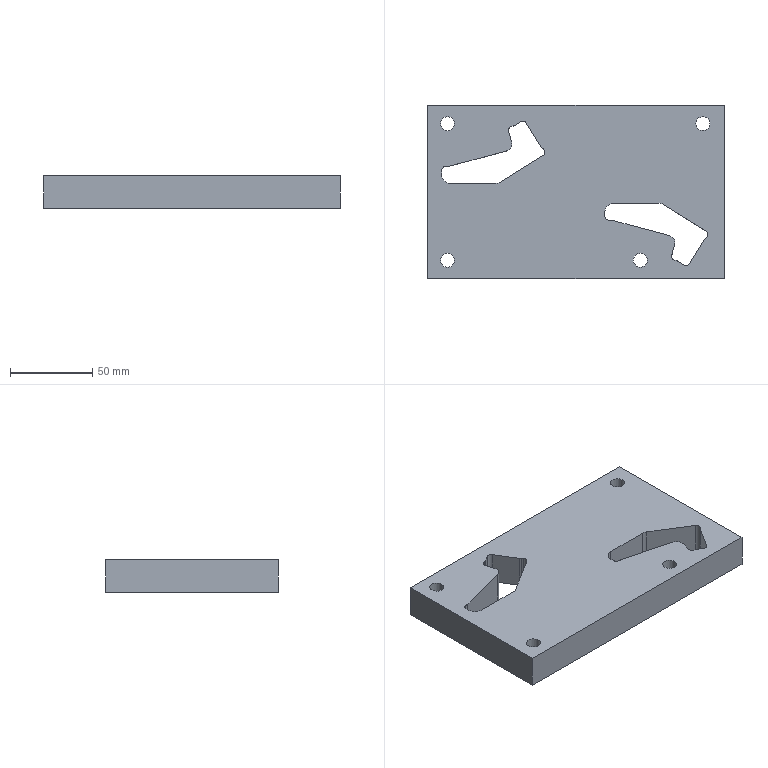Part | NX | features solid 2 | 1 solid | 62 faces | box 180 x 105 x 20 mm | volume 328547 mm3 | cylinder 32 | plane 28 | spline 2 | commonest cylinder face diameters 5 x12 3 x4 8.5 x4 9 x4 11 x4 14 x4